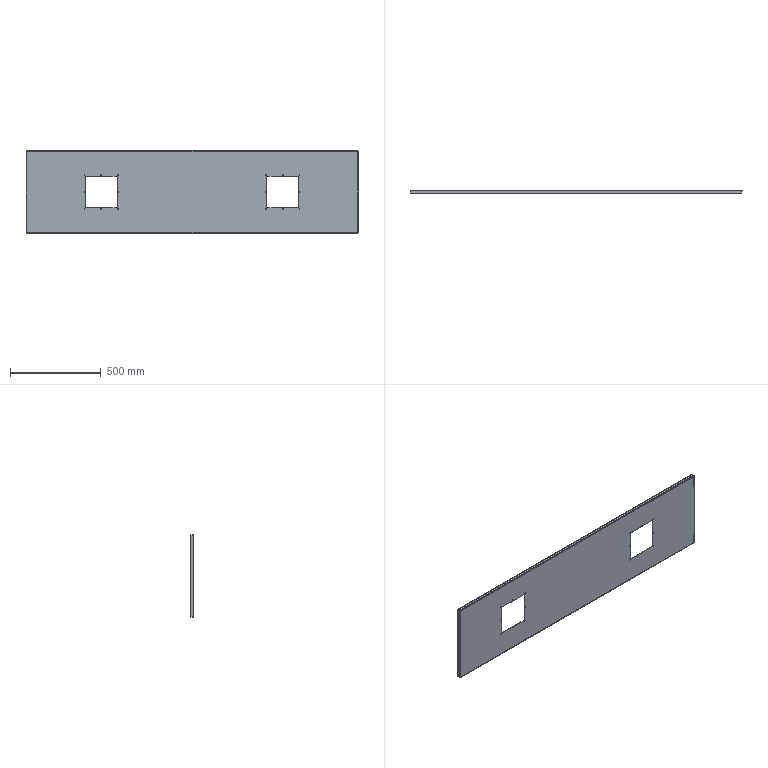Part | SolidWorks | features ICE 3, MirrorPattern 2, FlatPattern 1, SMBaseFlange 1, SMMiteredFlange 1, SheetMetal 1 | 1 solid | 122 faces | box 1828 x 20 x 453 mm | volume 1833705 mm3 | cylinder 60 | plane 46 | spline 16 | commonest cylinder face diameters 5 x32 7 x12 4 x8 8 x8